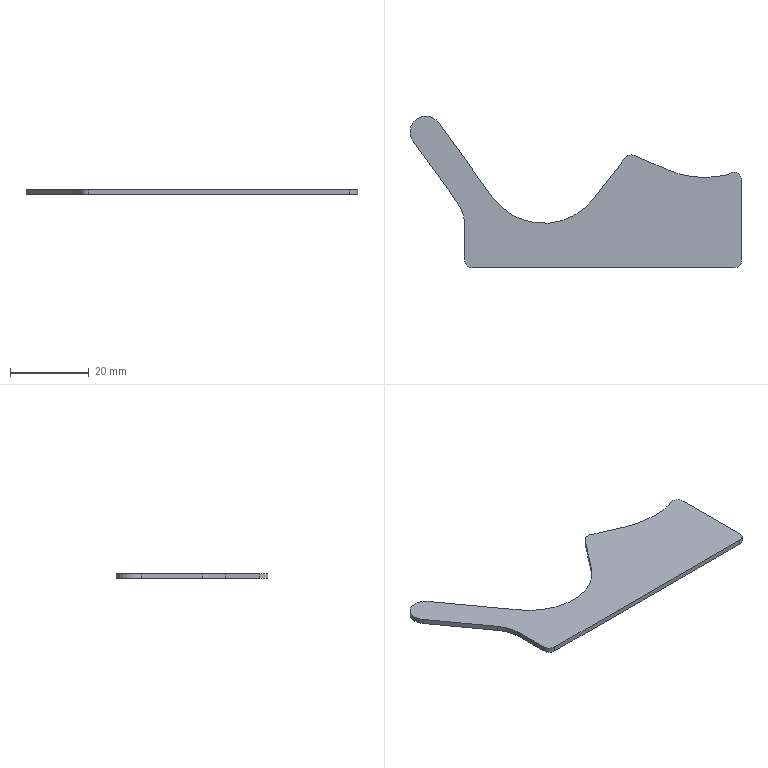Part | STEP file | gslz 2016.10.28-13_id194_x_t | 1 solid | 19 faces | box 84.166 x 38.478 x 1.25 mm | volume 1970 mm3 | cylinder 10 | plane 9 | commonest cylinder face diameters 4 x5 8 x1 20 x1 32 x1 46 x1 80 x1